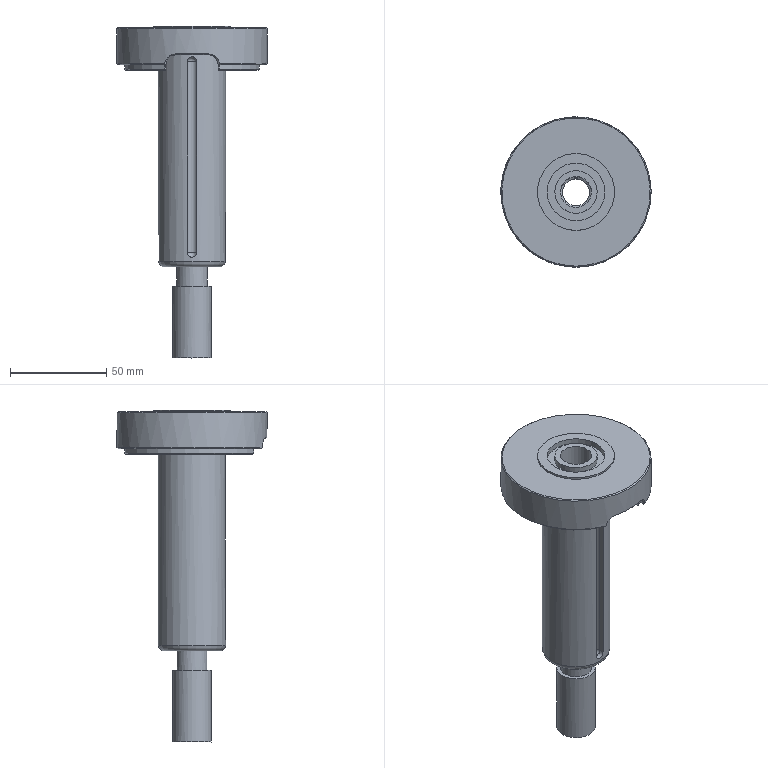Part | STEP file | solid 186 | 1 solid | 51 faces | box 78 x 78 x 172.328 mm | volume 163780 mm3 | plane 21 | cylinder 15 | spline 7 | cone 5 | sphere 2 | torus 1 | commonest cylinder face diameters 5 x3 10 x2 16 x2 14 x1 20 x1 22 x1